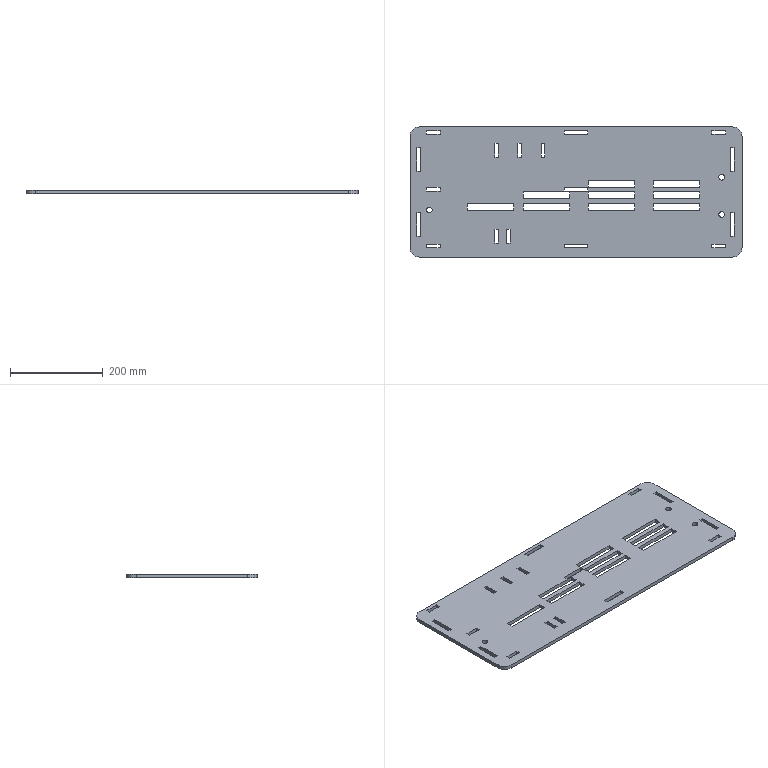Part | SolidWorks | features FlatPattern 1, SMBaseFlange 1, SheetMetal 1 | 1 solid | 120 faces | box 715 x 280 x 8 mm | volume 1446309 mm3 | plane 110 | cylinder 10 | commonest cylinder face diameters 12.5 x6 40 x4